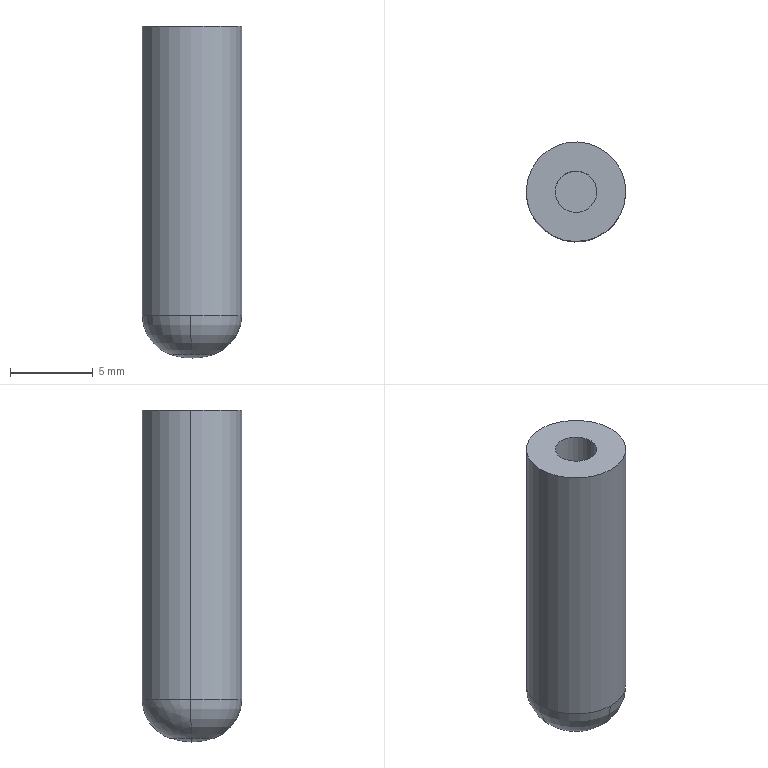Part | SolidWorks | features BaseBody 1 | 1 solid | 11 faces | box 6 x 6 x 20 mm | volume 493.517 mm3 | cylinder 4 | torus 2 | plane 2 | sphere 2 | spline 1 | commonest cylinder face diameters 2.5 x2 6 x2
STEP:
#1=CARTESIAN_POINT('',(-703.162,724.464,474.71));
#2=VERTEX_POINT('',#1);
#3=CARTESIAN_POINT('',(-704.463,725.829,474.71));
#4=VERTEX_POINT('',#3);
#5=CARTESIAN_POINT('',(-703.13,725.797,474.71));
#6=DIRECTION('',(0.,0.,-1.));
#7=DIRECTION('',(0.9997,-0.02414,0.));
#8=AXIS2_PLACEMENT_3D('',#5,#6,#7);
#9=CIRCLE('',#8,1.333);
#10=EDGE_CURVE('',#2,#4,#9,.T.);
#11=ORIENTED_EDGE('',*,*,#10,.F.);
#12=CARTESIAN_POINT('',(-703.202,722.798,477.068));
#13=VERTEX_POINT('',#12);
#14=CARTESIAN_POINT('',(-703.142,725.297,477.068));
#15=DIRECTION('',(-0.9997,0.02414,0.));
#16=DIRECTION('',(-0.02414,-0.9997,0.));
#17=AXIS2_PLACEMENT_3D('',#14,#15,#16);
#18=CIRCLE('',#17,2.5);
#19=EDGE_CURVE('',#2,#13,#18,.T.);
#20=ORIENTED_EDGE('',*,*,#19,.T.);
#21=CARTESIAN_POINT('',(-706.129,725.869,477.068));
#22=VERTEX_POINT('',#21);
#23=CARTESIAN_POINT('',(-703.13,725.797,477.068));
#24=DIRECTION('',(0.,0.,1.));
#25=DIRECTION('',(-0.9997,0.02414,0.));
#26=AXIS2_PLACEMENT_3D('',#23,#24,#25);
#27=CIRCLE('',#26,3.);
#28=EDGE_CURVE('',#22,#13,#27,.T.);
#29=ORIENTED_EDGE('',*,*,#28,.F.);
#30=CARTESIAN_POINT('',(-703.63,725.809,477.068));
#31=DIRECTION('',(0.02414,0.9997,0.));
#32=DIRECTION('',(-0.3332,0.008046,-0.9428));
#33=AXIS2_PLACEMENT_3D('',#30,#31,#32);
#34=CIRCLE('',#33,2.5);
#35=EDGE_CURVE('',#4,#22,#34,.T.);
#36=ORIENTED_EDGE('',*,*,#35,.F.);
#37=EDGE_LOOP('',(#11,#20,#29,#36));
#38=FACE_OUTER_BOUND('',#37,.T.);
#39=CARTESIAN_POINT('',(-703.13,725.797,477.068));
#40=DIRECTION('',(0.,0.,1.));
#41=DIRECTION('',(-0.02414,-0.9997,0.));
#42=AXIS2_PLACEMENT_3D('',#39,#40,#41);
#43=TOROIDAL_SURFACE('',#42,0.5,2.5);
#44=ADVANCED_FACE('',(#38),#43,.T.);
#45=CARTESIAN_POINT('',(-700.131,725.725,494.482));
#46=VERTEX_POINT('',#45);
#47=CARTESIAN_POINT('',(-706.129,725.869,494.482));
#48=VERTEX_POINT('',#47);
#49=CARTESIAN_POINT('',(-703.13,725.797,494.482));
#50=DIRECTION('',(0.,0.,-1.));
#51=DIRECTION('',(0.9997,-0.02414,0.));
#52=AXIS2_PLACEMENT_3D('',#49,#50,#51);
#53=CIRCLE('',#52,3.);
#54=EDGE_CURVE('',#46,#48,#53,.T.);
#55=ORIENTED_EDGE('',*,*,#54,.F.);
#56=CARTESIAN_POINT('',(-703.13,725.797,494.482));
#57=DIRECTION('',(0.,0.,-1.));
#58=DIRECTION('',(-0.9997,0.02414,0.));
#59=AXIS2_PLACEMENT_3D('',#56,#57,#58);
#60=CIRCLE('',#59,3.);
#61=EDGE_CURVE('',#48,#46,#60,.T.);
#62=ORIENTED_EDGE('',*,*,#61,.F.);
#63=EDGE_LOOP('',(#55,#62));
#64=FACE_OUTER_BOUND('',#63,.T.);
#65=CARTESIAN_POINT('',(-704.38,725.827,494.482));
#66=VERTEX_POINT('',#65);
#67=CARTESIAN_POINT('',(-701.88,725.767,494.482));
#68=VERTEX_POINT('',#67);
#69=CARTESIAN_POINT('',(-703.13,725.797,494.482));
#70=DIRECTION('',(0.,0.,1.));
#71=DIRECTION('',(-0.9997,0.02414,0.));
#72=AXIS2_PLACEMENT_3D('',#69,#70,#71);
#73=CIRCLE('',#72,1.25);
#74=EDGE_CURVE('',#66,#68,#73,.T.);
#75=ORIENTED_EDGE('',*,*,#74,.F.);
#76=CARTESIAN_POINT('',(-703.13,725.797,494.482));
#77=DIRECTION('',(0.,0.,1.));
#78=DIRECTION('',(0.9997,-0.02414,0.));
#79=AXIS2_PLACEMENT_3D('',#76,#77,#78);
#80=CIRCLE('',#79,1.25);
#81=EDGE_CURVE('',#68,#66,#80,.T.);
#82=ORIENTED_EDGE('',*,*,#81,.F.);
#83=EDGE_LOOP('',(#75,#82));
#84=FACE_BOUND('',#83,.T.);
#85=CARTESIAN_POINT('',(-619.649,574.908,494.482));
#86=DIRECTION('',(0.,0.,-1.));
#87=DIRECTION('',(0.9997,-0.02414,0.));
#88=AXIS2_PLACEMENT_3D('',#85,#86,#87);
#89=PLANE('',#88);
#90=ADVANCED_FACE('',(#64,#84),#89,.F.);
#91=ORIENTED_EDGE('',*,*,#61,.T.);
#92=CARTESIAN_POINT('',(-700.131,725.725,477.068));
#93=VERTEX_POINT('',#92);
#94=CARTESIAN_POINT('',(-700.131,725.725,494.482));
#95=DIRECTION('',(0.,0.,-1.));
#96=VECTOR('',#95,1000.);
#97=LINE('',#94,#96);
#98=EDGE_CURVE('',#46,#93,#97,.T.);
#99=ORIENTED_EDGE('',*,*,#98,.T.);
#100=CARTESIAN_POINT('',(-703.13,725.797,477.068));
#101=DIRECTION('',(0.,0.,1.));
#102=DIRECTION('',(0.9997,-0.02414,0.));
#103=AXIS2_PLACEMENT_3D('',#100,#101,#102);
#104=CIRCLE('',#103,3.);
#105=EDGE_CURVE('',#93,#22,#104,.T.);
#106=ORIENTED_EDGE('',*,*,#105,.T.);
#107=CARTESIAN_POINT('',(-706.129,725.869,477.068));
#108=DIRECTION('',(0.,0.,1.));
#109=VECTOR('',#108,1000.);
#110=LINE('',#107,#109);
#111=EDGE_CURVE('',#22,#48,#110,.T.);
#112=ORIENTED_EDGE('',*,*,#111,.T.);
#113=EDGE_LOOP('',(#91,#99,#106,#112));
#114=FACE_OUTER_BOUND('',#113,.T.);
#115=CARTESIAN_POINT('',(-703.13,725.797,494.482));
#116=DIRECTION('',(0.,0.,1.));
#117=DIRECTION('',(-0.9997,0.02414,0.));
#118=AXIS2_PLACEMENT_3D('',#115,#116,#117);
#119=CYLINDRICAL_SURFACE('',#118,3.);
#120=ADVANCED_FACE('',(#114),#119,.T.);
#121=ORIENTED_EDGE('',*,*,#54,.T.);
#122=ORIENTED_EDGE('',*,*,#111,.F.);
#123=ORIENTED_EDGE('',*,*,#28,.T.);
#124=CARTESIAN_POINT('',(-703.13,725.797,477.068));
#125=DIRECTION('',(0.,0.,1.));
#126=DIRECTION('',(-0.9997,0.02414,0.));
#127=AXIS2_PLACEMENT_3D('',#124,#125,#126);
#128=CIRCLE('',#127,3.);
#129=EDGE_CURVE('',#13,#93,#128,.T.);
#130=ORIENTED_EDGE('',*,*,#129,.T.);
#131=ORIENTED_EDGE('',*,*,#98,.F.);
#132=EDGE_LOOP('',(#121,#122,#123,#130,#131));
#133=FACE_OUTER_BOUND('',#132,.T.);
#134=CARTESIAN_POINT('',(-703.13,725.797,494.482));
#135=DIRECTION('',(0.,0.,1.));
#136=DIRECTION('',(-0.9997,0.02414,0.));
#137=AXIS2_PLACEMENT_3D('',#134,#135,#136);
#138=CYLINDRICAL_SURFACE('',#137,3.);
#139=ADVANCED_FACE('',(#133),#138,.T.);
#140=ORIENTED_EDGE('',*,*,#19,.F.);
#141=CARTESIAN_POINT('',(-701.797,725.765,474.71));
#142=VERTEX_POINT('',#141);
#143=CARTESIAN_POINT('',(-703.13,725.797,474.71));
#144=DIRECTION('',(0.,0.,-1.));
#145=DIRECTION('',(0.9997,-0.02414,0.));
#146=AXIS2_PLACEMENT_3D('',#143,#144,#145);
#147=CIRCLE('',#146,1.333);
#148=EDGE_CURVE('',#142,#2,#147,.T.);
#149=ORIENTED_EDGE('',*,*,#148,.F.);
#150=CARTESIAN_POINT('',(-702.63,725.785,477.068));
#151=DIRECTION('',(0.02414,0.9997,0.));
#152=DIRECTION('',(0.9997,-0.02414,0.));
#153=AXIS2_PLACEMENT_3D('',#150,#151,#152);
#154=CIRCLE('',#153,2.5);
#155=EDGE_CURVE('',#93,#142,#154,.T.);
#156=ORIENTED_EDGE('',*,*,#155,.F.);
#157=ORIENTED_EDGE('',*,*,#129,.F.);
#158=EDGE_LOOP('',(#140,#149,#156,#157));
#159=FACE_OUTER_BOUND('',#158,.T.);
#160=CARTESIAN_POINT('',(-703.13,725.797,477.068));
#161=DIRECTION('',(0.,0.,1.));
#162=DIRECTION('',(-0.02414,-0.9997,0.));
#163=AXIS2_PLACEMENT_3D('',#160,#161,#162);
#164=TOROIDAL_SURFACE('',#163,0.5,2.5);
#165=ADVANCED_FACE('',(#159),#164,.T.);
#166=ORIENTED_EDGE('',*,*,#105,.F.);
#167=ORIENTED_EDGE('',*,*,#155,.T.);
#168=CARTESIAN_POINT('',(-703.13,725.797,474.71));
#169=DIRECTION('',(0.,0.,-1.));
#170=DIRECTION('',(-0.9997,0.02414,0.));
#171=AXIS2_PLACEMENT_3D('',#168,#169,#170);
#172=CIRCLE('',#171,1.333);
#173=EDGE_CURVE('',#4,#142,#172,.T.);
#174=ORIENTED_EDGE('',*,*,#173,.F.);
#175=ORIENTED_EDGE('',*,*,#35,.T.);
#176=EDGE_LOOP('',(#166,#167,#174,#175));
#177=FACE_OUTER_BOUND('',#176,.T.);
#178=CARTESIAN_POINT('',(-701.86,725.686,474.691));
#179=CARTESIAN_POINT('',(-700.774,725.592,475.046));
#180=CARTESIAN_POINT('',(-700.114,725.534,475.983));
#181=CARTESIAN_POINT('',(-700.142,725.537,477.129));
#182=CARTESIAN_POINT('',(-701.792,726.468,474.691));
#183=CARTESIAN_POINT('',(-700.647,727.042,475.046));
#184=CARTESIAN_POINT('',(-699.952,727.39,475.983));
#185=CARTESIAN_POINT('',(-699.982,727.375,477.129));
#186=CARTESIAN_POINT('',(-702.315,727.053,474.691));
#187=CARTESIAN_POINT('',(-701.618,728.127,475.046));
#188=CARTESIAN_POINT('',(-701.194,728.779,475.983));
#189=CARTESIAN_POINT('',(-701.212,728.751,477.129));
#190=CARTESIAN_POINT('',(-703.099,727.072,474.691));
#191=CARTESIAN_POINT('',(-703.073,728.162,475.046));
#192=CARTESIAN_POINT('',(-703.057,728.824,475.983));
#193=CARTESIAN_POINT('',(-703.058,728.795,477.129));
#194=CARTESIAN_POINT('',(-703.884,727.091,474.691));
#195=CARTESIAN_POINT('',(-704.528,728.197,475.046));
#196=CARTESIAN_POINT('',(-704.92,728.869,475.983));
#197=CARTESIAN_POINT('',(-704.903,728.84,477.129));
#198=CARTESIAN_POINT('',(-704.434,726.532,474.691));
#199=CARTESIAN_POINT('',(-705.55,727.16,475.046));
#200=CARTESIAN_POINT('',(-706.227,727.542,475.983));
#201=CARTESIAN_POINT('',(-706.198,727.525,477.129));
#202=CARTESIAN_POINT('',(-704.404,725.748,474.691));
#203=CARTESIAN_POINT('',(-705.494,725.706,475.046));
#204=CARTESIAN_POINT('',(-706.155,725.68,475.983));
#205=CARTESIAN_POINT('',(-706.127,725.681,477.129));
#206=(BOUNDED_SURFACE()B_SPLINE_SURFACE(3,3,((#178,#179,#180,#181),(#182,#183,#184,#185),(#186,#187,#188,#189),(#190,#191,#192,#193),(#194,#195,#196,#197),(#198,#199,#200,#201),(#202,#203,#204,#205)),.UNSPECIFIED.,.F.,.F.,.T.)B_SPLINE_SURFACE_WITH_KNOTS((4,3,4),(4,4),(0.,0.5,1.),(0.,1.),.UNSPECIFIED.)GEOMETRIC_REPRESENTATION_ITEM()RATIONAL_B_SPLINE_SURFACE(((1.318,1.144,1.144,1.318),(1.041,0.9032,0.9032,1.041),(1.041,0.9032,0.9032,1.041),(1.318,1.144,1.144,1.318),(1.041,0.9032,0.9032,1.041),(1.041,0.9032,0.9032,1.041),(1.318,1.144,1.144,1.318)))REPRESENTATION_ITEM('')SURFACE());
#207=ADVANCED_FACE('',(#177),#206,.T.);
#208=CARTESIAN_POINT('',(-703.13,725.797,474.482));
#209=VERTEX_POINT('',#208);
#210=CARTESIAN_POINT('',(-703.13,725.797,478.482));
#211=DIRECTION('',(0.02414,0.9997,0.));
#212=DIRECTION('',(0.,0.,-1.));
#213=AXIS2_PLACEMENT_3D('',#210,#211,#212);
#214=CIRCLE('',#213,4.);
#215=EDGE_CURVE('',#209,#4,#214,.T.);
#216=ORIENTED_EDGE('',*,*,#215,.T.);
#217=ORIENTED_EDGE('',*,*,#173,.T.);
#218=CARTESIAN_POINT('',(-703.13,725.797,478.482));
#219=DIRECTION('',(0.02414,0.9997,0.));
#220=DIRECTION('',(0.3332,-0.008046,-0.9428));
#221=AXIS2_PLACEMENT_3D('',#218,#219,#220);
#222=CIRCLE('',#221,4.);
#223=EDGE_CURVE('',#142,#209,#222,.T.);
#224=ORIENTED_EDGE('',*,*,#223,.T.);
#225=EDGE_LOOP('',(#216,#217,#224));
#226=FACE_OUTER_BOUND('',#225,.T.);
#227=CARTESIAN_POINT('',(-703.13,725.797,478.482));
#228=DIRECTION('',(-0.02414,-0.9997,0.));
#229=DIRECTION('',(0.9997,-0.02414,0.));
#230=AXIS2_PLACEMENT_3D('',#227,#228,#229);
#231=SPHERICAL_SURFACE('',#230,4.);
#232=ADVANCED_FACE('',(#226),#231,.T.);
#233=ORIENTED_EDGE('',*,*,#223,.F.);
#234=ORIENTED_EDGE('',*,*,#148,.T.);
#235=ORIENTED_EDGE('',*,*,#10,.T.);
#236=ORIENTED_EDGE('',*,*,#215,.F.);
#237=EDGE_LOOP('',(#233,#234,#235,#236));
#238=FACE_OUTER_BOUND('',#237,.T.);
#239=CARTESIAN_POINT('',(-703.13,725.797,478.482));
#240=DIRECTION('',(-0.02414,-0.9997,0.));
#241=DIRECTION('',(0.9997,-0.02414,0.));
#242=AXIS2_PLACEMENT_3D('',#239,#240,#241);
#243=SPHERICAL_SURFACE('',#242,4.);
#244=ADVANCED_FACE('',(#238),#243,.T.);
#245=ORIENTED_EDGE('',*,*,#81,.T.);
#246=CARTESIAN_POINT('',(-704.38,725.827,484.482));
#247=VERTEX_POINT('',#246);
#248=CARTESIAN_POINT('',(-704.38,725.827,494.482));
#249=DIRECTION('',(0.,0.,-1.));
#250=VECTOR('',#249,1000.);
#251=LINE('',#248,#250);
#252=EDGE_CURVE('',#66,#247,#251,.T.);
#253=ORIENTED_EDGE('',*,*,#252,.T.);
#254=CARTESIAN_POINT('',(-701.88,725.767,484.482));
#255=VERTEX_POINT('',#254);
#256=CARTESIAN_POINT('',(-703.13,725.797,484.482));
#257=DIRECTION('',(0.,0.,-1.));
#258=DIRECTION('',(-0.9997,0.02414,0.));
#259=AXIS2_PLACEMENT_3D('',#256,#257,#258);
#260=CIRCLE('',#259,1.25);
#261=EDGE_CURVE('',#247,#255,#260,.T.);
#262=ORIENTED_EDGE('',*,*,#261,.T.);
#263=CARTESIAN_POINT('',(-701.88,725.767,484.482));
#264=DIRECTION('',(0.,0.,1.));
#265=VECTOR('',#264,1000.);
#266=LINE('',#263,#265);
#267=EDGE_CURVE('',#255,#68,#266,.T.);
#268=ORIENTED_EDGE('',*,*,#267,.T.);
#269=EDGE_LOOP('',(#245,#253,#262,#268));
#270=FACE_OUTER_BOUND('',#269,.T.);
#271=CARTESIAN_POINT('',(-703.13,725.797,494.482));
#272=DIRECTION('',(0.,0.,1.));
#273=DIRECTION('',(-0.9997,0.02414,0.));
#274=AXIS2_PLACEMENT_3D('',#271,#272,#273);
#275=CYLINDRICAL_SURFACE('',#274,1.25);
#276=ADVANCED_FACE('',(#270),#275,.F.);
#277=ORIENTED_EDGE('',*,*,#74,.T.);
#278=ORIENTED_EDGE('',*,*,#267,.F.);
#279=CARTESIAN_POINT('',(-703.13,725.797,484.482));
#280=DIRECTION('',(0.,0.,-1.));
#281=DIRECTION('',(0.9997,-0.02414,0.));
#282=AXIS2_PLACEMENT_3D('',#279,#280,#281);
#283=CIRCLE('',#282,1.25);
#284=EDGE_CURVE('',#255,#247,#283,.T.);
#285=ORIENTED_EDGE('',*,*,#284,.T.);
#286=ORIENTED_EDGE('',*,*,#252,.F.);
#287=EDGE_LOOP('',(#277,#278,#285,#286));
#288=FACE_OUTER_BOUND('',#287,.T.);
#289=CARTESIAN_POINT('',(-703.13,725.797,494.482));
#290=DIRECTION('',(0.,0.,1.));
#291=DIRECTION('',(-0.9997,0.02414,0.));
#292=AXIS2_PLACEMENT_3D('',#289,#290,#291);
#293=CYLINDRICAL_SURFACE('',#292,1.25);
#294=ADVANCED_FACE('',(#288),#293,.F.);
#295=ORIENTED_EDGE('',*,*,#284,.F.);
#296=ORIENTED_EDGE('',*,*,#261,.F.);
#297=EDGE_LOOP('',(#295,#296));
#298=FACE_OUTER_BOUND('',#297,.T.);
#299=CARTESIAN_POINT('',(-619.649,574.908,484.482));
#300=DIRECTION('',(0.,0.,1.));
#301=DIRECTION('',(-0.9997,0.02414,0.));
#302=AXIS2_PLACEMENT_3D('',#299,#300,#301);
#303=PLANE('',#302);
#304=ADVANCED_FACE('',(#298),#303,.T.);
#305=CLOSED_SHELL('',(#44,#90,#120,#139,#165,#207,#232,#244,#276,#294,#304));
#306=MANIFOLD_SOLID_BREP('',#305);
#307=CARTESIAN_POINT('',(0.,0.,0.));
#308=DIRECTION('',(0.,0.,1.));
#309=DIRECTION('',(1.,0.,0.));
#310=AXIS2_PLACEMENT_3D('',#307,#308,#309);
#311=(LENGTH_UNIT()NAMED_UNIT(*)SI_UNIT(.MILLI.,.METRE.));
#312=UNCERTAINTY_MEASURE_WITH_UNIT(LENGTH_MEASURE(0.00001),#311,'','');
#313=(NAMED_UNIT(*)PLANE_ANGLE_UNIT()SI_UNIT($,.RADIAN.));
#314=(NAMED_UNIT(*)SI_UNIT($,.STERADIAN.)SOLID_ANGLE_UNIT());
#315=(GEOMETRIC_REPRESENTATION_CONTEXT(3)GLOBAL_UNCERTAINTY_ASSIGNED_CONTEXT((#312))GLOBAL_UNIT_ASSIGNED_CONTEXT((#311,#313,#314))REPRESENTATION_CONTEXT('',''));
#316=ADVANCED_BREP_SHAPE_REPRESENTATION('',(#306,#310),#315);